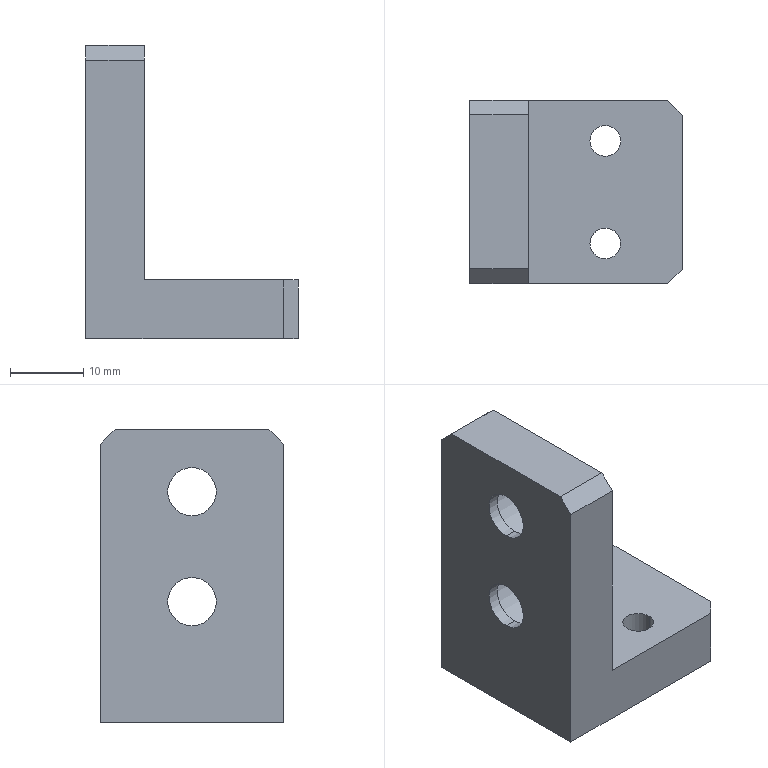Part | SolidWorks | features HoleWzd 2, Chamfer 1, Extrusion 1 | 1 solid | 26 faces | box 29 x 25 x 40 mm | volume 10588 mm3 | plane 14 | cylinder 12 | commonest cylinder face diameters 4.2 x4 6.6 x4 11 x4
STEP:
#1=CARTESIAN_POINT('',(-6.4,0.,-3.));
#2=VERTEX_POINT('',#1);
#3=CARTESIAN_POINT('',(-6.4,0.,-14.));
#4=VERTEX_POINT('',#3);
#5=CARTESIAN_POINT('',(-6.4,0.,-8.5));
#6=DIRECTION('',(1.,0.,0.));
#7=DIRECTION('',(0.,0.,-1.));
#8=AXIS2_PLACEMENT_3D('',#5,#6,#7);
#9=CIRCLE('',#8,5.5);
#10=EDGE_CURVE('',#2,#4,#9,.T.);
#11=ORIENTED_EDGE('',*,*,#10,.F.);
#12=CARTESIAN_POINT('',(0.,0.,-3.));
#13=VERTEX_POINT('',#12);
#14=CARTESIAN_POINT('',(0.,0.,-3.));
#15=DIRECTION('',(1.,0.,0.));
#16=VECTOR('',#15,1000.);
#17=LINE('',#14,#16);
#18=EDGE_CURVE('',#2,#13,#17,.T.);
#19=ORIENTED_EDGE('',*,*,#18,.T.);
#20=CARTESIAN_POINT('',(0.,0.,-14.));
#21=VERTEX_POINT('',#20);
#22=CARTESIAN_POINT('',(0.,0.,-8.5));
#23=DIRECTION('',(1.,0.,0.));
#24=DIRECTION('',(0.,0.,-1.));
#25=AXIS2_PLACEMENT_3D('',#22,#23,#24);
#26=CIRCLE('',#25,5.5);
#27=EDGE_CURVE('',#13,#21,#26,.T.);
#28=ORIENTED_EDGE('',*,*,#27,.T.);
#29=CARTESIAN_POINT('',(0.,0.,-14.));
#30=DIRECTION('',(1.,0.,0.));
#31=VECTOR('',#30,1000.);
#32=LINE('',#29,#31);
#33=EDGE_CURVE('',#4,#21,#32,.T.);
#34=ORIENTED_EDGE('',*,*,#33,.F.);
#35=EDGE_LOOP('',(#11,#19,#28,#34));
#36=FACE_OUTER_BOUND('',#35,.T.);
#37=CARTESIAN_POINT('',(0.,0.,-8.5));
#38=DIRECTION('',(1.,0.,0.));
#39=DIRECTION('',(0.,0.,-1.));
#40=AXIS2_PLACEMENT_3D('',#37,#38,#39);
#41=CYLINDRICAL_SURFACE('',#40,5.5);
#42=ADVANCED_FACE('',(#36),#41,.F.);
#43=CARTESIAN_POINT('',(-8.,0.,-5.2));
#44=VERTEX_POINT('',#43);
#45=CARTESIAN_POINT('',(-8.,0.,-11.8));
#46=VERTEX_POINT('',#45);
#47=CARTESIAN_POINT('',(-8.,0.,-8.5));
#48=DIRECTION('',(1.,0.,0.));
#49=DIRECTION('',(0.,0.,-1.));
#50=AXIS2_PLACEMENT_3D('',#47,#48,#49);
#51=CIRCLE('',#50,3.3);
#52=EDGE_CURVE('',#44,#46,#51,.T.);
#53=ORIENTED_EDGE('',*,*,#52,.F.);
#54=CARTESIAN_POINT('',(-6.4,0.,-5.2));
#55=VERTEX_POINT('',#54);
#56=CARTESIAN_POINT('',(0.,0.,-5.2));
#57=DIRECTION('',(1.,0.,0.));
#58=VECTOR('',#57,1000.);
#59=LINE('',#56,#58);
#60=EDGE_CURVE('',#44,#55,#59,.T.);
#61=ORIENTED_EDGE('',*,*,#60,.T.);
#62=CARTESIAN_POINT('',(-6.4,0.,-11.8));
#63=VERTEX_POINT('',#62);
#64=CARTESIAN_POINT('',(-6.4,0.,-8.5));
#65=DIRECTION('',(1.,0.,0.));
#66=DIRECTION('',(0.,0.,-1.));
#67=AXIS2_PLACEMENT_3D('',#64,#65,#66);
#68=CIRCLE('',#67,3.3);
#69=EDGE_CURVE('',#55,#63,#68,.T.);
#70=ORIENTED_EDGE('',*,*,#69,.T.);
#71=CARTESIAN_POINT('',(0.,0.,-11.8));
#72=DIRECTION('',(1.,0.,0.));
#73=VECTOR('',#72,1000.);
#74=LINE('',#71,#73);
#75=EDGE_CURVE('',#46,#63,#74,.T.);
#76=ORIENTED_EDGE('',*,*,#75,.F.);
#77=EDGE_LOOP('',(#53,#61,#70,#76));
#78=FACE_OUTER_BOUND('',#77,.T.);
#79=CARTESIAN_POINT('',(0.,0.,-8.5));
#80=DIRECTION('',(1.,0.,0.));
#81=DIRECTION('',(0.,0.,-1.));
#82=AXIS2_PLACEMENT_3D('',#79,#80,#81);
#83=CYLINDRICAL_SURFACE('',#82,3.3);
#84=ADVANCED_FACE('',(#78),#83,.F.);
#85=CARTESIAN_POINT('',(-6.4,0.,-18.));
#86=VERTEX_POINT('',#85);
#87=CARTESIAN_POINT('',(-6.4,0.,-29.));
#88=VERTEX_POINT('',#87);
#89=CARTESIAN_POINT('',(-6.4,0.,-23.5));
#90=DIRECTION('',(1.,0.,0.));
#91=DIRECTION('',(0.,0.,-1.));
#92=AXIS2_PLACEMENT_3D('',#89,#90,#91);
#93=CIRCLE('',#92,5.5);
#94=EDGE_CURVE('',#86,#88,#93,.T.);
#95=ORIENTED_EDGE('',*,*,#94,.F.);
#96=CARTESIAN_POINT('',(0.,0.,-18.));
#97=VERTEX_POINT('',#96);
#98=CARTESIAN_POINT('',(0.,0.,-18.));
#99=DIRECTION('',(1.,0.,0.));
#100=VECTOR('',#99,1000.);
#101=LINE('',#98,#100);
#102=EDGE_CURVE('',#86,#97,#101,.T.);
#103=ORIENTED_EDGE('',*,*,#102,.T.);
#104=CARTESIAN_POINT('',(0.,0.,-29.));
#105=VERTEX_POINT('',#104);
#106=CARTESIAN_POINT('',(0.,0.,-23.5));
#107=DIRECTION('',(1.,0.,0.));
#108=DIRECTION('',(0.,0.,-1.));
#109=AXIS2_PLACEMENT_3D('',#106,#107,#108);
#110=CIRCLE('',#109,5.5);
#111=EDGE_CURVE('',#97,#105,#110,.T.);
#112=ORIENTED_EDGE('',*,*,#111,.T.);
#113=CARTESIAN_POINT('',(0.,0.,-29.));
#114=DIRECTION('',(1.,0.,0.));
#115=VECTOR('',#114,1000.);
#116=LINE('',#113,#115);
#117=EDGE_CURVE('',#88,#105,#116,.T.);
#118=ORIENTED_EDGE('',*,*,#117,.F.);
#119=EDGE_LOOP('',(#95,#103,#112,#118));
#120=FACE_OUTER_BOUND('',#119,.T.);
#121=CARTESIAN_POINT('',(0.,0.,-23.5));
#122=DIRECTION('',(1.,0.,0.));
#123=DIRECTION('',(0.,0.,-1.));
#124=AXIS2_PLACEMENT_3D('',#121,#122,#123);
#125=CYLINDRICAL_SURFACE('',#124,5.5);
#126=ADVANCED_FACE('',(#120),#125,.F.);
#127=CARTESIAN_POINT('',(-8.,0.,-20.2));
#128=VERTEX_POINT('',#127);
#129=CARTESIAN_POINT('',(-8.,0.,-26.8));
#130=VERTEX_POINT('',#129);
#131=CARTESIAN_POINT('',(-8.,0.,-23.5));
#132=DIRECTION('',(1.,0.,0.));
#133=DIRECTION('',(0.,0.,-1.));
#134=AXIS2_PLACEMENT_3D('',#131,#132,#133);
#135=CIRCLE('',#134,3.3);
#136=EDGE_CURVE('',#128,#130,#135,.T.);
#137=ORIENTED_EDGE('',*,*,#136,.F.);
#138=CARTESIAN_POINT('',(-6.4,0.,-20.2));
#139=VERTEX_POINT('',#138);
#140=CARTESIAN_POINT('',(0.,0.,-20.2));
#141=DIRECTION('',(1.,0.,0.));
#142=VECTOR('',#141,1000.);
#143=LINE('',#140,#142);
#144=EDGE_CURVE('',#128,#139,#143,.T.);
#145=ORIENTED_EDGE('',*,*,#144,.T.);
#146=CARTESIAN_POINT('',(-6.4,0.,-26.8));
#147=VERTEX_POINT('',#146);
#148=CARTESIAN_POINT('',(-6.4,0.,-23.5));
#149=DIRECTION('',(1.,0.,0.));
#150=DIRECTION('',(0.,0.,-1.));
#151=AXIS2_PLACEMENT_3D('',#148,#149,#150);
#152=CIRCLE('',#151,3.3);
#153=EDGE_CURVE('',#139,#147,#152,.T.);
#154=ORIENTED_EDGE('',*,*,#153,.T.);
#155=CARTESIAN_POINT('',(0.,0.,-26.8));
#156=DIRECTION('',(1.,0.,0.));
#157=VECTOR('',#156,1000.);
#158=LINE('',#155,#157);
#159=EDGE_CURVE('',#130,#147,#158,.T.);
#160=ORIENTED_EDGE('',*,*,#159,.F.);
#161=EDGE_LOOP('',(#137,#145,#154,#160));
#162=FACE_OUTER_BOUND('',#161,.T.);
#163=CARTESIAN_POINT('',(0.,0.,-23.5));
#164=DIRECTION('',(1.,0.,0.));
#165=DIRECTION('',(0.,0.,-1.));
#166=AXIS2_PLACEMENT_3D('',#163,#164,#165);
#167=CYLINDRICAL_SURFACE('',#166,3.3);
#168=ADVANCED_FACE('',(#162),#167,.F.);
#169=CARTESIAN_POINT('',(8.4,7.,-40.));
#170=VERTEX_POINT('',#169);
#171=CARTESIAN_POINT('',(12.6,7.,-40.));
#172=VERTEX_POINT('',#171);
#173=CARTESIAN_POINT('',(10.5,7.,-40.));
#174=DIRECTION('',(0.,0.,1.));
#175=DIRECTION('',(1.,0.,0.));
#176=AXIS2_PLACEMENT_3D('',#173,#174,#175);
#177=CIRCLE('',#176,2.1);
#178=EDGE_CURVE('',#170,#172,#177,.T.);
#179=ORIENTED_EDGE('',*,*,#178,.F.);
#180=CARTESIAN_POINT('',(8.4,7.,-32.));
#181=VERTEX_POINT('',#180);
#182=CARTESIAN_POINT('',(8.4,7.,-32.));
#183=DIRECTION('',(0.,0.,1.));
#184=VECTOR('',#183,1000.);
#185=LINE('',#182,#184);
#186=EDGE_CURVE('',#170,#181,#185,.T.);
#187=ORIENTED_EDGE('',*,*,#186,.T.);
#188=CARTESIAN_POINT('',(12.6,7.,-32.));
#189=VERTEX_POINT('',#188);
#190=CARTESIAN_POINT('',(10.5,7.,-32.));
#191=DIRECTION('',(0.,0.,1.));
#192=DIRECTION('',(1.,0.,0.));
#193=AXIS2_PLACEMENT_3D('',#190,#191,#192);
#194=CIRCLE('',#193,2.1);
#195=EDGE_CURVE('',#181,#189,#194,.T.);
#196=ORIENTED_EDGE('',*,*,#195,.T.);
#197=CARTESIAN_POINT('',(12.6,7.,-32.));
#198=DIRECTION('',(0.,0.,1.));
#199=VECTOR('',#198,1000.);
#200=LINE('',#197,#199);
#201=EDGE_CURVE('',#172,#189,#200,.T.);
#202=ORIENTED_EDGE('',*,*,#201,.F.);
#203=EDGE_LOOP('',(#179,#187,#196,#202));
#204=FACE_OUTER_BOUND('',#203,.T.);
#205=CARTESIAN_POINT('',(10.5,7.,-32.));
#206=DIRECTION('',(0.,0.,1.));
#207=DIRECTION('',(1.,0.,0.));
#208=AXIS2_PLACEMENT_3D('',#205,#206,#207);
#209=CYLINDRICAL_SURFACE('',#208,2.1);
#210=ADVANCED_FACE('',(#204),#209,.F.);
#211=CARTESIAN_POINT('',(8.4,-7.,-40.));
#212=VERTEX_POINT('',#211);
#213=CARTESIAN_POINT('',(12.6,-7.,-40.));
#214=VERTEX_POINT('',#213);
#215=CARTESIAN_POINT('',(10.5,-7.,-40.));
#216=DIRECTION('',(0.,0.,1.));
#217=DIRECTION('',(1.,0.,0.));
#218=AXIS2_PLACEMENT_3D('',#215,#216,#217);
#219=CIRCLE('',#218,2.1);
#220=EDGE_CURVE('',#212,#214,#219,.T.);
#221=ORIENTED_EDGE('',*,*,#220,.F.);
#222=CARTESIAN_POINT('',(8.4,-7.,-32.));
#223=VERTEX_POINT('',#222);
#224=CARTESIAN_POINT('',(8.4,-7.,-32.));
#225=DIRECTION('',(0.,0.,1.));
#226=VECTOR('',#225,1000.);
#227=LINE('',#224,#226);
#228=EDGE_CURVE('',#212,#223,#227,.T.);
#229=ORIENTED_EDGE('',*,*,#228,.T.);
#230=CARTESIAN_POINT('',(12.6,-7.,-32.));
#231=VERTEX_POINT('',#230);
#232=CARTESIAN_POINT('',(10.5,-7.,-32.));
#233=DIRECTION('',(0.,0.,1.));
#234=DIRECTION('',(1.,0.,0.));
#235=AXIS2_PLACEMENT_3D('',#232,#233,#234);
#236=CIRCLE('',#235,2.1);
#237=EDGE_CURVE('',#223,#231,#236,.T.);
#238=ORIENTED_EDGE('',*,*,#237,.T.);
#239=CARTESIAN_POINT('',(12.6,-7.,-32.));
#240=DIRECTION('',(0.,0.,1.));
#241=VECTOR('',#240,1000.);
#242=LINE('',#239,#241);
#243=EDGE_CURVE('',#214,#231,#242,.T.);
#244=ORIENTED_EDGE('',*,*,#243,.F.);
#245=EDGE_LOOP('',(#221,#229,#238,#244));
#246=FACE_OUTER_BOUND('',#245,.T.);
#247=CARTESIAN_POINT('',(10.5,-7.,-32.));
#248=DIRECTION('',(0.,0.,1.));
#249=DIRECTION('',(1.,0.,0.));
#250=AXIS2_PLACEMENT_3D('',#247,#248,#249);
#251=CYLINDRICAL_SURFACE('',#250,2.1);
#252=ADVANCED_FACE('',(#246),#251,.F.);
#253=CARTESIAN_POINT('',(0.,10.5,0.));
#254=VERTEX_POINT('',#253);
#255=CARTESIAN_POINT('',(0.,-10.5,0.));
#256=VERTEX_POINT('',#255);
#257=CARTESIAN_POINT('',(0.,12.5,0.));
#258=DIRECTION('',(0.,-1.,0.));
#259=VECTOR('',#258,1000.);
#260=LINE('',#257,#259);
#261=EDGE_CURVE('',#254,#256,#260,.T.);
#262=ORIENTED_EDGE('',*,*,#261,.F.);
#263=CARTESIAN_POINT('',(-8.,10.5,0.));
#264=VERTEX_POINT('',#263);
#265=CARTESIAN_POINT('',(-8.,10.5,0.));
#266=DIRECTION('',(-1.,0.,0.));
#267=VECTOR('',#266,1000.);
#268=LINE('',#265,#267);
#269=EDGE_CURVE('',#254,#264,#268,.T.);
#270=ORIENTED_EDGE('',*,*,#269,.T.);
#271=CARTESIAN_POINT('',(-8.,-10.5,0.));
#272=VERTEX_POINT('',#271);
#273=CARTESIAN_POINT('',(-8.,12.5,0.));
#274=DIRECTION('',(0.,-1.,0.));
#275=VECTOR('',#274,1000.);
#276=LINE('',#273,#275);
#277=EDGE_CURVE('',#264,#272,#276,.T.);
#278=ORIENTED_EDGE('',*,*,#277,.T.);
#279=CARTESIAN_POINT('',(-8.,-10.5,0.));
#280=DIRECTION('',(1.,0.,0.));
#281=VECTOR('',#280,1000.);
#282=LINE('',#279,#281);
#283=EDGE_CURVE('',#272,#256,#282,.T.);
#284=ORIENTED_EDGE('',*,*,#283,.T.);
#285=EDGE_LOOP('',(#262,#270,#278,#284));
#286=FACE_OUTER_BOUND('',#285,.T.);
#287=CARTESIAN_POINT('',(-8.,12.5,0.));
#288=DIRECTION('',(0.,0.,-1.));
#289=DIRECTION('',(-1.,0.,0.));
#290=AXIS2_PLACEMENT_3D('',#287,#288,#289);
#291=PLANE('',#290);
#292=ADVANCED_FACE('',(#286),#291,.F.);
#293=CARTESIAN_POINT('',(0.,0.,-8.5));
#294=DIRECTION('',(1.,0.,0.));
#295=DIRECTION('',(0.,0.,-1.));
#296=AXIS2_PLACEMENT_3D('',#293,#294,#295);
#297=CIRCLE('',#296,5.5);
#298=EDGE_CURVE('',#21,#13,#297,.T.);
#299=ORIENTED_EDGE('',*,*,#298,.F.);
#300=ORIENTED_EDGE('',*,*,#27,.F.);
#301=EDGE_LOOP('',(#299,#300));
#302=FACE_BOUND('',#301,.T.);
#303=CARTESIAN_POINT('',(0.,0.,-23.5));
#304=DIRECTION('',(1.,0.,0.));
#305=DIRECTION('',(0.,0.,-1.));
#306=AXIS2_PLACEMENT_3D('',#303,#304,#305);
#307=CIRCLE('',#306,5.5);
#308=EDGE_CURVE('',#105,#97,#307,.T.);
#309=ORIENTED_EDGE('',*,*,#308,.F.);
#310=ORIENTED_EDGE('',*,*,#111,.F.);
#311=EDGE_LOOP('',(#309,#310));
#312=FACE_BOUND('',#311,.T.);
#313=CARTESIAN_POINT('',(0.,12.5,-2.));
#314=VERTEX_POINT('',#313);
#315=CARTESIAN_POINT('',(0.,12.5,-32.));
#316=VERTEX_POINT('',#315);
#317=CARTESIAN_POINT('',(0.,12.5,0.));
#318=DIRECTION('',(0.,0.,-1.));
#319=VECTOR('',#318,1000.);
#320=LINE('',#317,#319);
#321=EDGE_CURVE('',#314,#316,#320,.T.);
#322=ORIENTED_EDGE('',*,*,#321,.F.);
#323=CARTESIAN_POINT('',(0.,12.5,-2.));
#324=DIRECTION('',(0.,-0.7071,0.7071));
#325=VECTOR('',#324,1000.);
#326=LINE('',#323,#325);
#327=EDGE_CURVE('',#314,#254,#326,.T.);
#328=ORIENTED_EDGE('',*,*,#327,.T.);
#329=ORIENTED_EDGE('',*,*,#261,.T.);
#330=CARTESIAN_POINT('',(0.,-12.5,-2.));
#331=VERTEX_POINT('',#330);
#332=CARTESIAN_POINT('',(0.,-10.5,0.));
#333=DIRECTION('',(0.,-0.7071,-0.7071));
#334=VECTOR('',#333,1000.);
#335=LINE('',#332,#334);
#336=EDGE_CURVE('',#256,#331,#335,.T.);
#337=ORIENTED_EDGE('',*,*,#336,.T.);
#338=CARTESIAN_POINT('',(0.,-12.5,-32.));
#339=VERTEX_POINT('',#338);
#340=CARTESIAN_POINT('',(0.,-12.5,0.));
#341=DIRECTION('',(0.,0.,-1.));
#342=VECTOR('',#341,1000.);
#343=LINE('',#340,#342);
#344=EDGE_CURVE('',#331,#339,#343,.T.);
#345=ORIENTED_EDGE('',*,*,#344,.T.);
#346=CARTESIAN_POINT('',(0.,12.5,-32.));
#347=DIRECTION('',(0.,-1.,0.));
#348=VECTOR('',#347,1000.);
#349=LINE('',#346,#348);
#350=EDGE_CURVE('',#316,#339,#349,.T.);
#351=ORIENTED_EDGE('',*,*,#350,.F.);
#352=EDGE_LOOP('',(#322,#328,#329,#337,#345,#351));
#353=FACE_OUTER_BOUND('',#352,.T.);
#354=CARTESIAN_POINT('',(0.,12.5,0.));
#355=DIRECTION('',(-1.,0.,0.));
#356=DIRECTION('',(0.,0.,1.));
#357=AXIS2_PLACEMENT_3D('',#354,#355,#356);
#358=PLANE('',#357);
#359=ADVANCED_FACE('',(#302,#312,#353),#358,.F.);
#360=CARTESIAN_POINT('',(10.5,7.,-32.));
#361=DIRECTION('',(0.,0.,1.));
#362=DIRECTION('',(1.,0.,0.));
#363=AXIS2_PLACEMENT_3D('',#360,#361,#362);
#364=CIRCLE('',#363,2.1);
#365=EDGE_CURVE('',#189,#181,#364,.T.);
#366=ORIENTED_EDGE('',*,*,#365,.F.);
#367=ORIENTED_EDGE('',*,*,#195,.F.);
#368=EDGE_LOOP('',(#366,#367));
#369=FACE_BOUND('',#368,.T.);
#370=CARTESIAN_POINT('',(10.5,-7.,-32.));
#371=DIRECTION('',(0.,0.,1.));
#372=DIRECTION('',(1.,0.,0.));
#373=AXIS2_PLACEMENT_3D('',#370,#371,#372);
#374=CIRCLE('',#373,2.1);
#375=EDGE_CURVE('',#231,#223,#374,.T.);
#376=ORIENTED_EDGE('',*,*,#375,.F.);
#377=ORIENTED_EDGE('',*,*,#237,.F.);
#378=EDGE_LOOP('',(#376,#377));
#379=FACE_BOUND('',#378,.T.);
#380=CARTESIAN_POINT('',(19.,-12.5,-32.));
#381=VERTEX_POINT('',#380);
#382=CARTESIAN_POINT('',(0.,-12.5,-32.));
#383=DIRECTION('',(1.,0.,0.));
#384=VECTOR('',#383,1000.);
#385=LINE('',#382,#384);
#386=EDGE_CURVE('',#339,#381,#385,.T.);
#387=ORIENTED_EDGE('',*,*,#386,.T.);
#388=CARTESIAN_POINT('',(21.,-10.5,-32.));
#389=VERTEX_POINT('',#388);
#390=CARTESIAN_POINT('',(21.,-10.5,-32.));
#391=DIRECTION('',(0.7071,0.7071,0.));
#392=VECTOR('',#391,1000.);
#393=LINE('',#390,#392);
#394=EDGE_CURVE('',#381,#389,#393,.T.);
#395=ORIENTED_EDGE('',*,*,#394,.T.);
#396=CARTESIAN_POINT('',(21.,10.5,-32.));
#397=VERTEX_POINT('',#396);
#398=CARTESIAN_POINT('',(21.,12.5,-32.));
#399=DIRECTION('',(0.,-1.,0.));
#400=VECTOR('',#399,1000.);
#401=LINE('',#398,#400);
#402=EDGE_CURVE('',#397,#389,#401,.T.);
#403=ORIENTED_EDGE('',*,*,#402,.F.);
#404=CARTESIAN_POINT('',(19.,12.5,-32.));
#405=VERTEX_POINT('',#404);
#406=CARTESIAN_POINT('',(19.,12.5,-32.));
#407=DIRECTION('',(-0.7071,0.7071,0.));
#408=VECTOR('',#407,1000.);
#409=LINE('',#406,#408);
#410=EDGE_CURVE('',#397,#405,#409,.T.);
#411=ORIENTED_EDGE('',*,*,#410,.T.);
#412=CARTESIAN_POINT('',(0.,12.5,-32.));
#413=DIRECTION('',(1.,0.,0.));
#414=VECTOR('',#413,1000.);
#415=LINE('',#412,#414);
#416=EDGE_CURVE('',#316,#405,#415,.T.);
#417=ORIENTED_EDGE('',*,*,#416,.F.);
#418=ORIENTED_EDGE('',*,*,#350,.T.);
#419=EDGE_LOOP('',(#387,#395,#403,#411,#417,#418));
#420=FACE_OUTER_BOUND('',#419,.T.);
#421=CARTESIAN_POINT('',(0.,12.5,-32.));
#422=DIRECTION('',(0.,0.,-1.));
#423=DIRECTION('',(-1.,0.,0.));
#424=AXIS2_PLACEMENT_3D('',#421,#422,#423);
#425=PLANE('',#424);
#426=ADVANCED_FACE('',(#369,#379,#420),#425,.F.);
#427=ORIENTED_EDGE('',*,*,#402,.T.);
#428=CARTESIAN_POINT('',(21.,-10.5,-40.));
#429=VERTEX_POINT('',#428);
#430=CARTESIAN_POINT('',(21.,-10.5,-32.));
#431=DIRECTION('',(0.,0.,-1.));
#432=VECTOR('',#431,1000.);
#433=LINE('',#430,#432);
#434=EDGE_CURVE('',#389,#429,#433,.T.);
#435=ORIENTED_EDGE('',*,*,#434,.T.);
#436=CARTESIAN_POINT('',(21.,10.5,-40.));
#437=VERTEX_POINT('',#436);
#438=CARTESIAN_POINT('',(21.,12.5,-40.));
#439=DIRECTION('',(0.,-1.,0.));
#440=VECTOR('',#439,1000.);
#441=LINE('',#438,#440);
#442=EDGE_CURVE('',#437,#429,#441,.T.);
#443=ORIENTED_EDGE('',*,*,#442,.F.);
#444=CARTESIAN_POINT('',(21.,10.5,-32.));
#445=DIRECTION('',(0.,0.,1.));
#446=VECTOR('',#445,1000.);
#447=LINE('',#444,#446);
#448=EDGE_CURVE('',#437,#397,#447,.T.);
#449=ORIENTED_EDGE('',*,*,#448,.T.);
#450=EDGE_LOOP('',(#427,#435,#443,#449));
#451=FACE_OUTER_BOUND('',#450,.T.);
#452=CARTESIAN_POINT('',(21.,12.5,-32.));
#453=DIRECTION('',(-1.,0.,0.));
#454=DIRECTION('',(0.,0.,1.));
#455=AXIS2_PLACEMENT_3D('',#452,#453,#454);
#456=PLANE('',#455);
#457=ADVANCED_FACE('',(#451),#456,.F.);
#458=CARTESIAN_POINT('',(10.5,7.,-40.));
#459=DIRECTION('',(0.,0.,1.));
#460=DIRECTION('',(1.,0.,0.));
#461=AXIS2_PLACEMENT_3D('',#458,#459,#460);
#462=CIRCLE('',#461,2.1);
#463=EDGE_CURVE('',#172,#170,#462,.T.);
#464=ORIENTED_EDGE('',*,*,#463,.T.);
#465=ORIENTED_EDGE('',*,*,#178,.T.);
#466=EDGE_LOOP('',(#464,#465));
#467=FACE_BOUND('',#466,.T.);
#468=CARTESIAN_POINT('',(10.5,-7.,-40.));
#469=DIRECTION('',(0.,0.,1.));
#470=DIRECTION('',(1.,0.,0.));
#471=AXIS2_PLACEMENT_3D('',#468,#469,#470);
#472=CIRCLE('',#471,2.1);
#473=EDGE_CURVE('',#214,#212,#472,.T.);
#474=ORIENTED_EDGE('',*,*,#473,.T.);
#475=ORIENTED_EDGE('',*,*,#220,.T.);
#476=EDGE_LOOP('',(#474,#475));
#477=FACE_BOUND('',#476,.T.);
#478=ORIENTED_EDGE('',*,*,#442,.T.);
#479=CARTESIAN_POINT('',(19.,-12.5,-40.));
#480=VERTEX_POINT('',#479);
#481=CARTESIAN_POINT('',(21.,-10.5,-40.));
#482=DIRECTION('',(-0.7071,-0.7071,0.));
#483=VECTOR('',#482,1000.);
#484=LINE('',#481,#483);
#485=EDGE_CURVE('',#429,#480,#484,.T.);
#486=ORIENTED_EDGE('',*,*,#485,.T.);
#487=CARTESIAN_POINT('',(-8.,-12.5,-40.));
#488=VERTEX_POINT('',#487);
#489=CARTESIAN_POINT('',(21.,-12.5,-40.));
#490=DIRECTION('',(-1.,0.,0.));
#491=VECTOR('',#490,1000.);
#492=LINE('',#489,#491);
#493=EDGE_CURVE('',#480,#488,#492,.T.);
#494=ORIENTED_EDGE('',*,*,#493,.T.);
#495=CARTESIAN_POINT('',(-8.,12.5,-40.));
#496=VERTEX_POINT('',#495);
#497=CARTESIAN_POINT('',(-8.,12.5,-40.));
#498=DIRECTION('',(0.,-1.,0.));
#499=VECTOR('',#498,1000.);
#500=LINE('',#497,#499);
#501=EDGE_CURVE('',#496,#488,#500,.T.);
#502=ORIENTED_EDGE('',*,*,#501,.F.);
#503=CARTESIAN_POINT('',(19.,12.5,-40.));
#504=VERTEX_POINT('',#503);
#505=CARTESIAN_POINT('',(21.,12.5,-40.));
#506=DIRECTION('',(-1.,0.,0.));
#507=VECTOR('',#506,1000.);
#508=LINE('',#505,#507);
#509=EDGE_CURVE('',#504,#496,#508,.T.);
#510=ORIENTED_EDGE('',*,*,#509,.F.);
#511=CARTESIAN_POINT('',(19.,12.5,-40.));
#512=DIRECTION('',(0.7071,-0.7071,0.));
#513=VECTOR('',#512,1000.);
#514=LINE('',#511,#513);
#515=EDGE_CURVE('',#504,#437,#514,.T.);
#516=ORIENTED_EDGE('',*,*,#515,.T.);
#517=EDGE_LOOP('',(#478,#486,#494,#502,#510,#516));
#518=FACE_OUTER_BOUND('',#517,.T.);
#519=CARTESIAN_POINT('',(21.,12.5,-40.));
#520=DIRECTION('',(0.,0.,1.));
#521=DIRECTION('',(1.,0.,0.));
#522=AXIS2_PLACEMENT_3D('',#519,#520,#521);
#523=PLANE('',#522);
#524=ADVANCED_FACE('',(#467,#477,#518),#523,.F.);
#525=CARTESIAN_POINT('',(-8.,0.,-8.5));
#526=DIRECTION('',(1.,0.,0.));
#527=DIRECTION('',(0.,0.,-1.));
#528=AXIS2_PLACEMENT_3D('',#525,#526,#527);
#529=CIRCLE('',#528,3.3);
#530=EDGE_CURVE('',#46,#44,#529,.T.);
#531=ORIENTED_EDGE('',*,*,#530,.T.);
#532=ORIENTED_EDGE('',*,*,#52,.T.);
#533=EDGE_LOOP('',(#531,#532));
#534=FACE_BOUND('',#533,.T.);
#535=CARTESIAN_POINT('',(-8.,0.,-23.5));
#536=DIRECTION('',(1.,0.,0.));
#537=DIRECTION('',(0.,0.,-1.));
#538=AXIS2_PLACEMENT_3D('',#535,#536,#537);
#539=CIRCLE('',#538,3.3);
#540=EDGE_CURVE('',#130,#128,#539,.T.);
#541=ORIENTED_EDGE('',*,*,#540,.T.);
#542=ORIENTED_EDGE('',*,*,#136,.T.);
#543=EDGE_LOOP('',(#541,#542));
#544=FACE_BOUND('',#543,.T.);
#545=ORIENTED_EDGE('',*,*,#277,.F.);
#546=CARTESIAN_POINT('',(-8.,12.5,-2.));
#547=VERTEX_POINT('',#546);
#548=CARTESIAN_POINT('',(-8.,12.5,-2.));
#549=DIRECTION('',(0.,0.7071,-0.7071));
#550=VECTOR('',#549,1000.);
#551=LINE('',#548,#550);
#552=EDGE_CURVE('',#264,#547,#551,.T.);
#553=ORIENTED_EDGE('',*,*,#552,.T.);
#554=CARTESIAN_POINT('',(-8.,12.5,-40.));
#555=DIRECTION('',(0.,0.,1.));
#556=VECTOR('',#555,1000.);
#557=LINE('',#554,#556);
#558=EDGE_CURVE('',#496,#547,#557,.T.);
#559=ORIENTED_EDGE('',*,*,#558,.F.);
#560=ORIENTED_EDGE('',*,*,#501,.T.);
#561=CARTESIAN_POINT('',(-8.,-12.5,-2.));
#562=VERTEX_POINT('',#561);
#563=CARTESIAN_POINT('',(-8.,-12.5,-40.));
#564=DIRECTION('',(0.,0.,1.));
#565=VECTOR('',#564,1000.);
#566=LINE('',#563,#565);
#567=EDGE_CURVE('',#488,#562,#566,.T.);
#568=ORIENTED_EDGE('',*,*,#567,.T.);
#569=CARTESIAN_POINT('',(-8.,-10.5,0.));
#570=DIRECTION('',(0.,0.7071,0.7071));
#571=VECTOR('',#570,1000.);
#572=LINE('',#569,#571);
#573=EDGE_CURVE('',#562,#272,#572,.T.);
#574=ORIENTED_EDGE('',*,*,#573,.T.);
#575=EDGE_LOOP('',(#545,#553,#559,#560,#568,#574));
#576=FACE_OUTER_BOUND('',#575,.T.);
#577=CARTESIAN_POINT('',(-8.,12.5,-40.));
#578=DIRECTION('',(1.,0.,0.));
#579=DIRECTION('',(0.,0.,-1.));
#580=AXIS2_PLACEMENT_3D('',#577,#578,#579);
#581=PLANE('',#580);
#582=ADVANCED_FACE('',(#534,#544,#576),#581,.F.);
#583=ORIENTED_EDGE('',*,*,#558,.T.);
#584=CARTESIAN_POINT('',(0.,12.5,-2.));
#585=DIRECTION('',(1.,0.,0.));
#586=VECTOR('',#585,1000.);
#587=LINE('',#584,#586);
#588=EDGE_CURVE('',#547,#314,#587,.T.);
#589=ORIENTED_EDGE('',*,*,#588,.T.);
#590=ORIENTED_EDGE('',*,*,#321,.T.);
#591=ORIENTED_EDGE('',*,*,#416,.T.);
#592=CARTESIAN_POINT('',(19.,12.5,-40.));
#593=DIRECTION('',(0.,0.,-1.));
#594=VECTOR('',#593,1000.);
#595=LINE('',#592,#594);
#596=EDGE_CURVE('',#405,#504,#595,.T.);
#597=ORIENTED_EDGE('',*,*,#596,.T.);
#598=ORIENTED_EDGE('',*,*,#509,.T.);
#599=EDGE_LOOP('',(#583,#589,#590,#591,#597,#598));
#600=FACE_OUTER_BOUND('',#599,.T.);
#601=CARTESIAN_POINT('',(0.,12.5,0.));
#602=DIRECTION('',(0.,1.,0.));
#603=DIRECTION('',(0.,0.,1.));
#604=AXIS2_PLACEMENT_3D('',#601,#602,#603);
#605=PLANE('',#604);
#606=ADVANCED_FACE('',(#600),#605,.T.);
#607=ORIENTED_EDGE('',*,*,#344,.F.);
#608=CARTESIAN_POINT('',(0.,-12.5,-2.));
#609=DIRECTION('',(-1.,0.,0.));
#610=VECTOR('',#609,1000.);
#611=LINE('',#608,#610);
#612=EDGE_CURVE('',#331,#562,#611,.T.);
#613=ORIENTED_EDGE('',*,*,#612,.T.);
#614=ORIENTED_EDGE('',*,*,#567,.F.);
#615=ORIENTED_EDGE('',*,*,#493,.F.);
#616=CARTESIAN_POINT('',(19.,-12.5,0.));
#617=DIRECTION('',(0.,0.,1.));
#618=VECTOR('',#617,1000.);
#619=LINE('',#616,#618);
#620=EDGE_CURVE('',#480,#381,#619,.T.);
#621=ORIENTED_EDGE('',*,*,#620,.T.);
#622=ORIENTED_EDGE('',*,*,#386,.F.);
#623=EDGE_LOOP('',(#607,#613,#614,#615,#621,#622));
#624=FACE_OUTER_BOUND('',#623,.T.);
#625=CARTESIAN_POINT('',(0.,-12.5,0.));
#626=DIRECTION('',(0.,1.,0.));
#627=DIRECTION('',(0.,0.,1.));
#628=AXIS2_PLACEMENT_3D('',#625,#626,#627);
#629=PLANE('',#628);
#630=ADVANCED_FACE('',(#624),#629,.F.);
#631=ORIENTED_EDGE('',*,*,#228,.F.);
#632=ORIENTED_EDGE('',*,*,#473,.F.);
#633=ORIENTED_EDGE('',*,*,#243,.T.);
#634=ORIENTED_EDGE('',*,*,#375,.T.);
#635=EDGE_LOOP('',(#631,#632,#633,#634));
#636=FACE_OUTER_BOUND('',#635,.T.);
#637=CARTESIAN_POINT('',(10.5,-7.,-32.));
#638=DIRECTION('',(0.,0.,1.));
#639=DIRECTION('',(1.,0.,0.));
#640=AXIS2_PLACEMENT_3D('',#637,#638,#639);
#641=CYLINDRICAL_SURFACE('',#640,2.1);
#642=ADVANCED_FACE('',(#636),#641,.F.);
#643=ORIENTED_EDGE('',*,*,#186,.F.);
#644=ORIENTED_EDGE('',*,*,#463,.F.);
#645=ORIENTED_EDGE('',*,*,#201,.T.);
#646=ORIENTED_EDGE('',*,*,#365,.T.);
#647=EDGE_LOOP('',(#643,#644,#645,#646));
#648=FACE_OUTER_BOUND('',#647,.T.);
#649=CARTESIAN_POINT('',(10.5,7.,-32.));
#650=DIRECTION('',(0.,0.,1.));
#651=DIRECTION('',(1.,0.,0.));
#652=AXIS2_PLACEMENT_3D('',#649,#650,#651);
#653=CYLINDRICAL_SURFACE('',#652,2.1);
#654=ADVANCED_FACE('',(#648),#653,.F.);
#655=ORIENTED_EDGE('',*,*,#144,.F.);
#656=ORIENTED_EDGE('',*,*,#540,.F.);
#657=ORIENTED_EDGE('',*,*,#159,.T.);
#658=CARTESIAN_POINT('',(-6.4,0.,-23.5));
#659=DIRECTION('',(1.,0.,0.));
#660=DIRECTION('',(0.,0.,-1.));
#661=AXIS2_PLACEMENT_3D('',#658,#659,#660);
#662=CIRCLE('',#661,3.3);
#663=EDGE_CURVE('',#147,#139,#662,.T.);
#664=ORIENTED_EDGE('',*,*,#663,.T.);
#665=EDGE_LOOP('',(#655,#656,#657,#664));
#666=FACE_OUTER_BOUND('',#665,.T.);
#667=CARTESIAN_POINT('',(0.,0.,-23.5));
#668=DIRECTION('',(1.,0.,0.));
#669=DIRECTION('',(0.,0.,-1.));
#670=AXIS2_PLACEMENT_3D('',#667,#668,#669);
#671=CYLINDRICAL_SURFACE('',#670,3.3);
#672=ADVANCED_FACE('',(#666),#671,.F.);
#673=ORIENTED_EDGE('',*,*,#663,.F.);
#674=ORIENTED_EDGE('',*,*,#153,.F.);
#675=EDGE_LOOP('',(#673,#674));
#676=FACE_BOUND('',#675,.T.);
#677=CARTESIAN_POINT('',(-6.4,0.,-23.5));
#678=DIRECTION('',(1.,0.,0.));
#679=DIRECTION('',(0.,0.,-1.));
#680=AXIS2_PLACEMENT_3D('',#677,#678,#679);
#681=CIRCLE('',#680,5.5);
#682=EDGE_CURVE('',#88,#86,#681,.T.);
#683=ORIENTED_EDGE('',*,*,#682,.T.);
#684=ORIENTED_EDGE('',*,*,#94,.T.);
#685=EDGE_LOOP('',(#683,#684));
#686=FACE_OUTER_BOUND('',#685,.T.);
#687=CARTESIAN_POINT('',(-6.4,3.3,-23.5));
#688=DIRECTION('',(-1.,0.,0.));
#689=DIRECTION('',(0.,0.,1.));
#690=AXIS2_PLACEMENT_3D('',#687,#688,#689);
#691=PLANE('',#690);
#692=ADVANCED_FACE('',(#676,#686),#691,.F.);
#693=ORIENTED_EDGE('',*,*,#102,.F.);
#694=ORIENTED_EDGE('',*,*,#682,.F.);
#695=ORIENTED_EDGE('',*,*,#117,.T.);
#696=ORIENTED_EDGE('',*,*,#308,.T.);
#697=EDGE_LOOP('',(#693,#694,#695,#696));
#698=FACE_OUTER_BOUND('',#697,.T.);
#699=CARTESIAN_POINT('',(0.,0.,-23.5));
#700=DIRECTION('',(1.,0.,0.));
#701=DIRECTION('',(0.,0.,-1.));
#702=AXIS2_PLACEMENT_3D('',#699,#700,#701);
#703=CYLINDRICAL_SURFACE('',#702,5.5);
#704=ADVANCED_FACE('',(#698),#703,.F.);
#705=ORIENTED_EDGE('',*,*,#60,.F.);
#706=ORIENTED_EDGE('',*,*,#530,.F.);
#707=ORIENTED_EDGE('',*,*,#75,.T.);
#708=CARTESIAN_POINT('',(-6.4,0.,-8.5));
#709=DIRECTION('',(1.,0.,0.));
#710=DIRECTION('',(0.,0.,-1.));
#711=AXIS2_PLACEMENT_3D('',#708,#709,#710);
#712=CIRCLE('',#711,3.3);
#713=EDGE_CURVE('',#63,#55,#712,.T.);
#714=ORIENTED_EDGE('',*,*,#713,.T.);
#715=EDGE_LOOP('',(#705,#706,#707,#714));
#716=FACE_OUTER_BOUND('',#715,.T.);
#717=CARTESIAN_POINT('',(0.,0.,-8.5));
#718=DIRECTION('',(1.,0.,0.));
#719=DIRECTION('',(0.,0.,-1.));
#720=AXIS2_PLACEMENT_3D('',#717,#718,#719);
#721=CYLINDRICAL_SURFACE('',#720,3.3);
#722=ADVANCED_FACE('',(#716),#721,.F.);
#723=ORIENTED_EDGE('',*,*,#713,.F.);
#724=ORIENTED_EDGE('',*,*,#69,.F.);
#725=EDGE_LOOP('',(#723,#724));
#726=FACE_BOUND('',#725,.T.);
#727=CARTESIAN_POINT('',(-6.4,0.,-8.5));
#728=DIRECTION('',(1.,0.,0.));
#729=DIRECTION('',(0.,0.,-1.));
#730=AXIS2_PLACEMENT_3D('',#727,#728,#729);
#731=CIRCLE('',#730,5.5);
#732=EDGE_CURVE('',#4,#2,#731,.T.);
#733=ORIENTED_EDGE('',*,*,#732,.T.);
#734=ORIENTED_EDGE('',*,*,#10,.T.);
#735=EDGE_LOOP('',(#733,#734));
#736=FACE_OUTER_BOUND('',#735,.T.);
#737=CARTESIAN_POINT('',(-6.4,3.3,-8.5));
#738=DIRECTION('',(-1.,0.,0.));
#739=DIRECTION('',(0.,0.,1.));
#740=AXIS2_PLACEMENT_3D('',#737,#738,#739);
#741=PLANE('',#740);
#742=ADVANCED_FACE('',(#726,#736),#741,.F.);
#743=ORIENTED_EDGE('',*,*,#18,.F.);
#744=ORIENTED_EDGE('',*,*,#732,.F.);
#745=ORIENTED_EDGE('',*,*,#33,.T.);
#746=ORIENTED_EDGE('',*,*,#298,.T.);
#747=EDGE_LOOP('',(#743,#744,#745,#746));
#748=FACE_OUTER_BOUND('',#747,.T.);
#749=CARTESIAN_POINT('',(0.,0.,-8.5));
#750=DIRECTION('',(1.,0.,0.));
#751=DIRECTION('',(0.,0.,-1.));
#752=AXIS2_PLACEMENT_3D('',#749,#750,#751);
#753=CYLINDRICAL_SURFACE('',#752,5.5);
#754=ADVANCED_FACE('',(#748),#753,.F.);
#755=ORIENTED_EDGE('',*,*,#552,.F.);
#756=ORIENTED_EDGE('',*,*,#269,.F.);
#757=ORIENTED_EDGE('',*,*,#327,.F.);
#758=ORIENTED_EDGE('',*,*,#588,.F.);
#759=EDGE_LOOP('',(#755,#756,#757,#758));
#760=FACE_OUTER_BOUND('',#759,.T.);
#761=CARTESIAN_POINT('',(0.,12.5,-2.));
#762=DIRECTION('',(0.,0.7071,0.7071));
#763=DIRECTION('',(-1.,0.,0.));
#764=AXIS2_PLACEMENT_3D('',#761,#762,#763);
#765=PLANE('',#764);
#766=ADVANCED_FACE('',(#760),#765,.T.);
#767=ORIENTED_EDGE('',*,*,#573,.F.);
#768=ORIENTED_EDGE('',*,*,#612,.F.);
#769=ORIENTED_EDGE('',*,*,#336,.F.);
#770=ORIENTED_EDGE('',*,*,#283,.F.);
#771=EDGE_LOOP('',(#767,#768,#769,#770));
#772=FACE_OUTER_BOUND('',#771,.T.);
#773=CARTESIAN_POINT('',(-8.,-10.5,0.));
#774=DIRECTION('',(0.,0.7071,-0.7071));
#775=DIRECTION('',(1.,0.,0.));
#776=AXIS2_PLACEMENT_3D('',#773,#774,#775);
#777=PLANE('',#776);
#778=ADVANCED_FACE('',(#772),#777,.F.);
#779=ORIENTED_EDGE('',*,*,#394,.F.);
#780=ORIENTED_EDGE('',*,*,#620,.F.);
#781=ORIENTED_EDGE('',*,*,#485,.F.);
#782=ORIENTED_EDGE('',*,*,#434,.F.);
#783=EDGE_LOOP('',(#779,#780,#781,#782));
#784=FACE_OUTER_BOUND('',#783,.T.);
#785=CARTESIAN_POINT('',(21.,-10.5,-32.));
#786=DIRECTION('',(-0.7071,0.7071,0.));
#787=DIRECTION('',(0.,0.,-1.));
#788=AXIS2_PLACEMENT_3D('',#785,#786,#787);
#789=PLANE('',#788);
#790=ADVANCED_FACE('',(#784),#789,.F.);
#791=ORIENTED_EDGE('',*,*,#410,.F.);
#792=ORIENTED_EDGE('',*,*,#448,.F.);
#793=ORIENTED_EDGE('',*,*,#515,.F.);
#794=ORIENTED_EDGE('',*,*,#596,.F.);
#795=EDGE_LOOP('',(#791,#792,#793,#794));
#796=FACE_OUTER_BOUND('',#795,.T.);
#797=CARTESIAN_POINT('',(19.,12.5,0.));
#798=DIRECTION('',(0.7071,0.7071,0.));
#799=DIRECTION('',(0.,0.,1.));
#800=AXIS2_PLACEMENT_3D('',#797,#798,#799);
#801=PLANE('',#800);
#802=ADVANCED_FACE('',(#796),#801,.T.);
#803=CLOSED_SHELL('',(#42,#84,#126,#168,#210,#252,#292,#359,#426,#457,#524,#582,#606,#630,#642,#654,#672,#692,#704,#722,#742,#754,#766,#778,#790,#802));
#804=MANIFOLD_SOLID_BREP('',#803);
#805=CARTESIAN_POINT('',(0.,0.,0.));
#806=DIRECTION('',(0.,0.,1.));
#807=DIRECTION('',(1.,0.,0.));
#808=AXIS2_PLACEMENT_3D('',#805,#806,#807);
#809=(LENGTH_UNIT()NAMED_UNIT(*)SI_UNIT(.MILLI.,.METRE.));
#810=UNCERTAINTY_MEASURE_WITH_UNIT(LENGTH_MEASURE(0.00001),#809,'','');
#811=(NAMED_UNIT(*)PLANE_ANGLE_UNIT()SI_UNIT($,.RADIAN.));
#812=(NAMED_UNIT(*)SI_UNIT($,.STERADIAN.)SOLID_ANGLE_UNIT());
#813=(GEOMETRIC_REPRESENTATION_CONTEXT(3)GLOBAL_UNCERTAINTY_ASSIGNED_CONTEXT((#810))GLOBAL_UNIT_ASSIGNED_CONTEXT((#809,#811,#812))REPRESENTATION_CONTEXT('',''));
#814=ADVANCED_BREP_SHAPE_REPRESENTATION('',(#804,#808),#813);